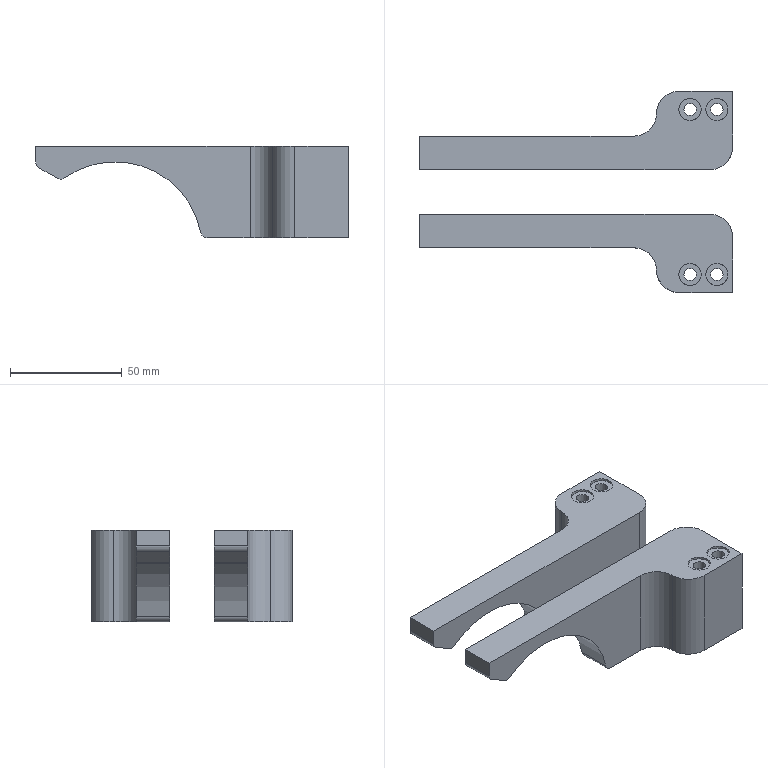NC program | NX | posted with a generic post | part box 140 x 90 x 41 mm
Lines 5013 to 5311 of 28919:
(ZLEVEL_PROFILE_COPY_COPY_COPY_1_COPY_COPY_COPY , TOOL : D12JING)
N10000 T11 M6
N10002 G54
N10004 G17 G0 G90 X62.666 Y-26.918 S9500 M3
N10006 G43 Z30. H11
N10008 Z-13.667
N10010 G94 G1 X61.039 Y-24.1 F1000.
N10012 G3 X60. Y-23.5 R1.2
N10014 G1 X-70. F1200.
N10016 G2 X-76. Y-17.5 R6.
N10018 G1 Y-2.5
N10020 G2 X-70. Y3.5 R6.
N10022 G1 X26.
N10024 G3 X30. Y7.5 R4.
N10026 G2 X46. Y23.5 R16.
N10028 G1 X70.
N10030 G2 X76. Y17.5 R6.
N10032 G1 Y-7.5
N10034 G2 X60. Y-23.5 R16.
N10036 G3 X58.961 Y-24.1 R1.2
N10038 G1 X57.229 Y-27.1
N10040 G0 X62.666 Y-26.918 Z-27.333
N10042 G1 X61.039 Y-24.1 F1000.
N10044 G3 X60. Y-23.5 R1.2
N10046 G1 X-70. F1200.
N10048 G2 X-76. Y-17.5 R6.
N10050 G1 Y-2.5
N10052 G2 X-70. Y3.5 R6.
N10054 G1 X26.
N10056 G3 X30. Y7.5 R4.
N10058 G2 X46. Y23.5 R16.
N10060 G1 X70.
N10062 G2 X76. Y17.5 R6.
N10064 G1 Y-7.5
N10066 G2 X60. Y-23.5 R16.
N10068 G3 X58.961 Y-24.1 R1.2
N10070 G1 X57.229 Y-27.1
N10072 G0 X62.666 Y-26.918 Z-41.
N10074 G1 X61.039 Y-24.1 F1000.
N10076 G3 X60. Y-23.5 R1.2
N10078 G1 X-70. F1200.
N10080 G2 X-76. Y-17.5 R6.
N10082 G1 Y-2.5
N10084 G2 X-70. Y3.5 R6.
N10086 G1 X26.
N10088 G3 X30. Y7.5 R4.
N10090 G2 X46. Y23.5 R16.
N10092 G1 X70.
N10094 G2 X76. Y17.5 R6.
N10096 G1 Y-7.5
N10098 G2 X60. Y-23.5 R16.
N10100 G3 X58.961 Y-24.1 R1.2
N10102 G1 X57.229 Y-27.1
N10104 G0 Z30.
(ZLEVEL_PROFILE , TOOL : D12JING)
N10106 X76.231 Y9.503
N10108 Z0.
N10110 G1 Z-0.95 F1650.
N10112 X75.389 Y9.498
N10114 X70.335
N10116 X70. Y9.5
N10118 X44.9
N10120 G3 X44.8 Y9.4 R0.1
N10122 X44.9 Y9.3 R0.1
N10124 G1 X70.
N10126 X70.335 Y9.302
N10128 X75.389
N10130 X76.231 Y9.297
N10132 G3 X76.532 Y9.375 R0.6
N10134 G0 X76.231 Y9.503
N10136 G1 Z-1.9
N10138 X75.389 Y9.498
N10140 X70.335
N10142 X70. Y9.5
N10144 X44.9
N10146 G3 X44.8 Y9.4 R0.1
N10148 X44.9 Y9.3 R0.1
N10150 G1 X70.
N10152 X70.335 Y9.302
N10154 X75.389
N10156 X76.231 Y9.297
N10158 G3 X76.532 Y9.375 R0.6
N10160 G0 X76.231 Y9.503
N10162 G1 Z-2.85
N10164 X75.389 Y9.497
N10166 X70.335
N10168 X70. Y9.5
N10170 X44.9
N10172 G3 X44.8 Y9.4 R0.1
N10174 X44.9 Y9.3 R0.1
N10176 G1 X70.
N10178 X70.335 Y9.303
N10180 X75.389
N10182 X76.231 Y9.297
N10184 G3 X76.532 Y9.376 R0.6
N10186 G0 X76.231 Y9.503
N10188 G1 Z-3.8
N10190 X75.389 Y9.497
N10192 X70.335
N10194 X70. Y9.5
N10196 X44.9
N10198 G3 X44.8 Y9.4 R0.1
N10200 X44.9 Y9.3 R0.1
N10202 G1 X70.
N10204 X70.335 Y9.303
N10206 X75.389
N10208 X76.231 Y9.297
N10210 G3 X76.532 Y9.376 R0.6
N10212 G0 X76.231 Y9.503
N10214 G1 Z-4.75
N10216 X75.389 Y9.497
N10218 X70.335
N10220 X70. Y9.5
N10222 X44.9
N10224 G3 X44.8 Y9.4 R0.1
N10226 X44.9 Y9.3 R0.1
N10228 G1 X70.
N10230 X70.335 Y9.303
N10232 X75.389
N10234 X76.231 Y9.297
N10236 G3 X76.532 Y9.376 R0.6
N10238 G0 X76.231 Y9.502
N10240 G1 Z-5.7
N10242 X75.389 Y9.497
N10244 X70.335
N10246 X70. Y9.5
N10248 X44.9
N10250 G3 X44.8 Y9.4 R0.1
N10252 X44.9 Y9.3 R0.1
N10254 G1 X70.
N10256 X70.335 Y9.303
N10258 X75.389
N10260 X76.231 Y9.298
N10262 G3 X76.532 Y9.376 R0.6
N10264 G0 X76.231 Y9.502
N10266 G1 Z-6.65
N10268 X75.389 Y9.496
N10270 X70.335
N10272 X70. Y9.5
N10274 X44.9
N10276 G3 X44.8 Y9.4 R0.1
N10278 X44.9 Y9.3 R0.1
N10280 G1 X70.
N10282 X70.335 Y9.304
N10284 X75.389
N10286 X76.231 Y9.298
N10288 G3 X76.532 Y9.376 R0.6
N10290 G0 X76.231 Y9.502
N10292 G1 Z-7.6
N10294 X75.389 Y9.496
N10296 X70.335
N10298 X70. Y9.5
N10300 X44.9
N10302 G3 X44.8 Y9.4 R0.1
N10304 X44.9 Y9.3 R0.1
N10306 G1 X70.
N10308 X70.335 Y9.304
N10310 X75.389
N10312 X76.231 Y9.298
N10314 G3 X76.532 Y9.376 R0.6
N10316 G0 X76.231 Y9.502
N10318 G1 Z-8.55
N10320 X75.389 Y9.496
N10322 X70.335
N10324 X70. Y9.5
N10326 X44.9
N10328 G3 X44.8 Y9.4 R0.1
N10330 X44.9 Y9.3 R0.1
N10332 G1 X70.
N10334 X70.335 Y9.304
N10336 X75.389
N10338 X76.231 Y9.298
N10340 G3 X76.532 Y9.376 R0.6
N10342 G0 X76.231 Y9.502
N10344 G1 Z-9.5
N10346 X75.389 Y9.496
N10348 X70.335
N10350 X70. Y9.5
N10352 X44.9
N10354 G3 X44.8 Y9.4 R0.1
N10356 X44.9 Y9.3 R0.1
N10358 G1 X70.
N10360 X70.335 Y9.304
N10362 X75.389
N10364 X76.231 Y9.298
N10366 G3 X76.532 Y9.376 R0.6
N10368 G0 X76.231 Y9.502
N10370 G1 Z-10.45
N10372 X75.389 Y9.495
N10374 X70.335
N10376 X70. Y9.5
N10378 X44.9
N10380 G3 X44.8 Y9.4 R0.1
N10382 X44.9 Y9.3 R0.1
N10384 G1 X70.
N10386 X70.335 Y9.305
N10388 X75.389
N10390 X76.231 Y9.298
N10392 G3 X76.532 Y9.376 R0.6
N10394 G0 X76.231 Y9.502
N10396 G1 Z-11.4
N10398 X75.389 Y9.495
N10400 X70.335
N10402 X70. Y9.5
N10404 X44.9
N10406 G3 X44.8 Y9.4 R0.1
N10408 X44.9 Y9.3 R0.1
N10410 G1 X70.
N10412 X70.335 Y9.305
N10414 X75.389
N10416 X76.231 Y9.298
N10418 G3 X76.532 Y9.376 R0.6
N10420 G0 X76.231 Y9.501
N10422 G1 Z-12.35
N10424 X75.389 Y9.495
N10426 X70.335
N10428 X70. Y9.5
N10430 X44.9
N10432 G3 X44.8 Y9.4 R0.1
N10434 X44.9 Y9.3 R0.1
N10436 G1 X70.
N10438 X70.335 Y9.305
N10440 X75.389
N10442 X76.231 Y9.299
N10444 G3 X76.532 Y9.377 R0.6
N10446 G0 X76.231 Y9.501
N10448 G1 Z-13.3
N10450 X75.389 Y9.495
N10452 X70.335
N10454 X70. Y9.5
N10456 X44.9
N10458 G3 X44.8 Y9.4 R0.1
N10460 X44.9 Y9.3 R0.1
N10462 G1 X70.
N10464 X70.335 Y9.305
N10466 X75.389
N10468 X76.231 Y9.299
N10470 G3 X76.532 Y9.377 R0.6
N10472 G0 X76.231 Y9.501
N10474 G1 Z-14.25
N10476 X75.389 Y9.494
N10478 X70.335
N10480 X70. Y9.5
N10482 X44.9
N10484 G3 X44.8 Y9.4 R0.1
N10486 X44.9 Y9.3 R0.1
N10488 G1 X70.
N10490 X70.335 Y9.306
N10492 X75.389
N10494 X76.231 Y9.299
N10496 G3 X76.532 Y9.377 R0.6
N10498 G0 X76.231 Y9.501
N10500 G1 Z-15.2
N10502 X75.389 Y9.494
N10504 X70.335
N10506 X70. Y9.5
N10508 X44.9
N10510 G3 X44.8 Y9.4 R0.1
N10512 X44.9 Y9.3 R0.1
N10514 G1 X70.
N10516 X70.335 Y9.306
N10518 X75.389
N10520 X76.231 Y9.299
N10522 G3 X76.532 Y9.377 R0.6
N10524 G0 Z30.
N10526 M5
(PLANAR_MILL , TOOL : D6A45)
N10528 T07 M6
N10530 G54
N10532 G17 G0 G90 X7.883 Y-0.682 S9500 M3
N10534 G43 Z30. H7
N10536 Z0.
N10538 G94 G1 Z-1. F1250.
N10540 G3 X8.031 Y-1.6 R1.
N10542 G1 X26.
N10544 G3 X35.1 Y7.5 R9.1
N10546 G2 X46. Y18.4 R10.9
N10548 G1 X69.9
N10550 G2 X70.9 Y17.4 R1.
N10552 G1 Y15.6
N10554 G2 X69.9 Y14.6 R1.
N10556 G1 X44.9
N10558 G3 X39.7 Y9.4 R5.2
N10560 X44.9 Y4.2 R5.2
N10562 G1 X69.9
N10564 G2 X70.9 Y3.2 R1.
N10566 G1 Y-7.5
N10568 G2 X60. Y-18.4 R10.9
N10570 G1 X8.031
N10572 G3 X7.883 Y-19.318 R1.
N10574 G1 Z0.
N10576 G0 Z30.
N10578 M5